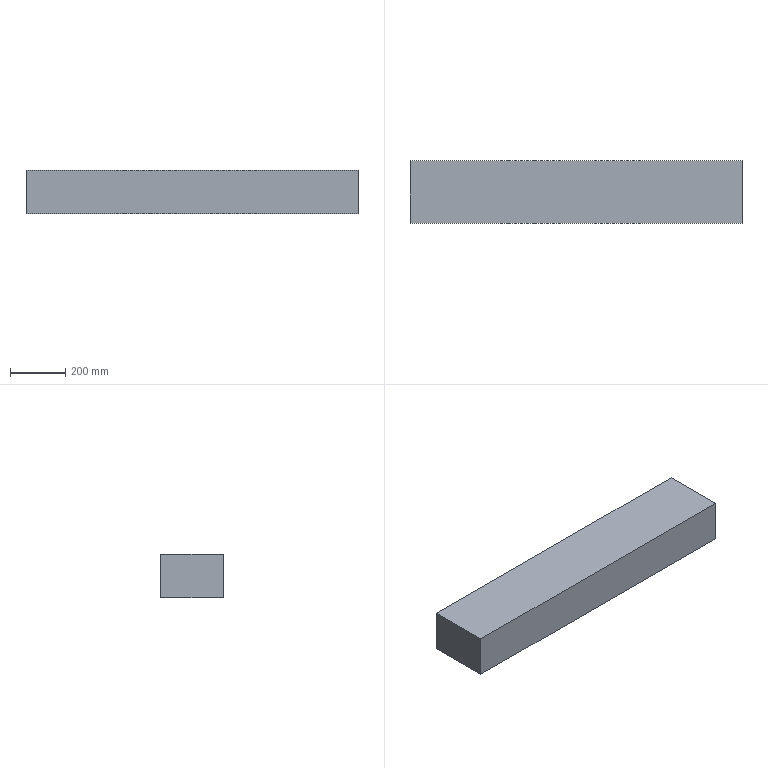Part | STEP file | 1 solid | 44 faces | box 1200 x 227 x 156.72 mm | volume 9554357 mm3 | plane 44